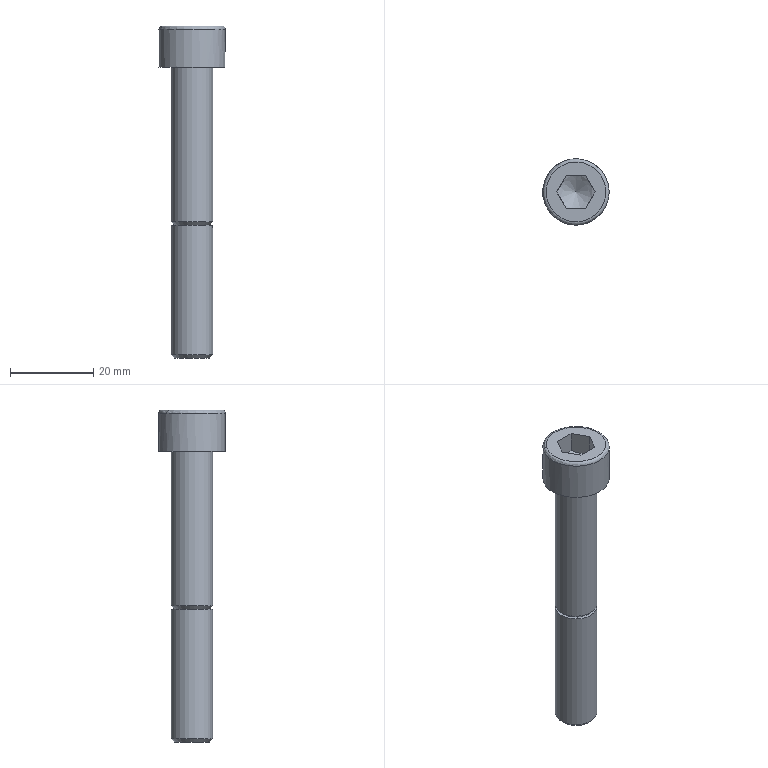Part | STEP file | 1_39 | 1 solid | 17 faces | box 16 x 16 x 80 mm | volume 7147 mm3 | plane 10 | cylinder 3 | cone 3 | torus 1 | commonest cylinder face diameters 10 x2 16 x1